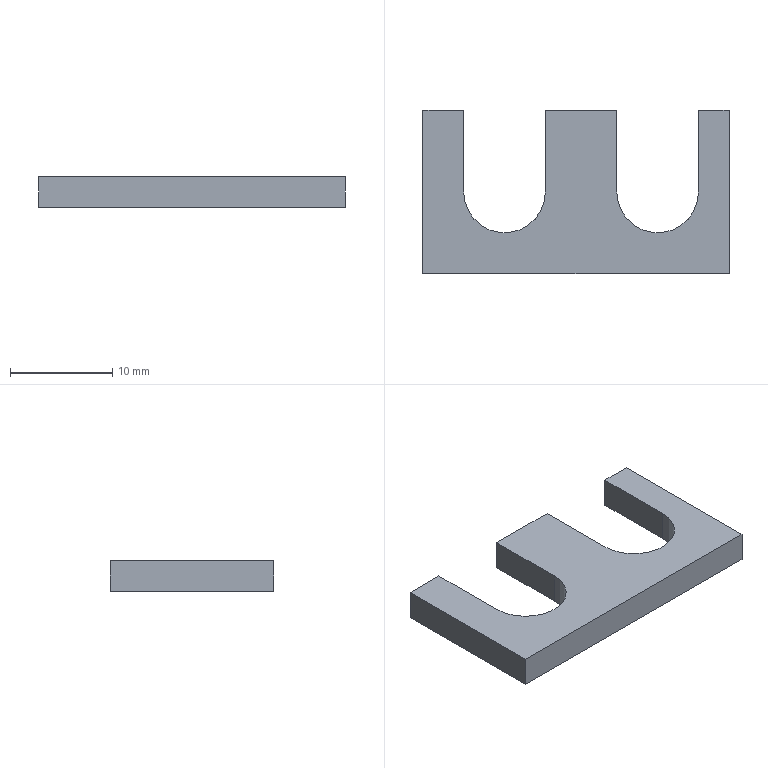Part | SolidWorks | features Extrusion 1 | 1 solid | 14 faces | box 30 x 16 x 3 mm | volume 905.204 mm3 | plane 12 | cylinder 2 | commonest cylinder face diameters 8 x2
STEP:
#1=CARTESIAN_POINT('',(0.,16.,0.));
#2=VERTEX_POINT('',#1);
#3=CARTESIAN_POINT('',(0.,0.,0.));
#4=VERTEX_POINT('',#3);
#5=CARTESIAN_POINT('',(0.,0.,0.));
#6=DIRECTION('',(0.,-1.,0.));
#7=VECTOR('',#6,1000.);
#8=LINE('',#5,#7);
#9=EDGE_CURVE('',#2,#4,#8,.T.);
#10=ORIENTED_EDGE('',*,*,#9,.T.);
#11=CARTESIAN_POINT('',(0.,0.,3.));
#12=VERTEX_POINT('',#11);
#13=CARTESIAN_POINT('',(0.,0.,3.));
#14=DIRECTION('',(0.,0.,-1.));
#15=VECTOR('',#14,1000.);
#16=LINE('',#13,#15);
#17=EDGE_CURVE('',#12,#4,#16,.T.);
#18=ORIENTED_EDGE('',*,*,#17,.F.);
#19=CARTESIAN_POINT('',(0.,16.,3.));
#20=VERTEX_POINT('',#19);
#21=CARTESIAN_POINT('',(0.,0.,3.));
#22=DIRECTION('',(0.,-1.,0.));
#23=VECTOR('',#22,1000.);
#24=LINE('',#21,#23);
#25=EDGE_CURVE('',#20,#12,#24,.T.);
#26=ORIENTED_EDGE('',*,*,#25,.F.);
#27=CARTESIAN_POINT('',(0.,16.,3.));
#28=DIRECTION('',(0.,0.,-1.));
#29=VECTOR('',#28,1000.);
#30=LINE('',#27,#29);
#31=EDGE_CURVE('',#20,#2,#30,.T.);
#32=ORIENTED_EDGE('',*,*,#31,.T.);
#33=EDGE_LOOP('',(#10,#18,#26,#32));
#34=FACE_OUTER_BOUND('',#33,.T.);
#35=CARTESIAN_POINT('',(0.,0.,3.));
#36=DIRECTION('',(1.,0.,0.));
#37=DIRECTION('',(0.,0.,-1.));
#38=AXIS2_PLACEMENT_3D('',#35,#36,#37);
#39=PLANE('',#38);
#40=ADVANCED_FACE('',(#34),#39,.F.);
#41=CARTESIAN_POINT('',(30.,0.,0.));
#42=VERTEX_POINT('',#41);
#43=CARTESIAN_POINT('',(0.,0.,0.));
#44=DIRECTION('',(1.,0.,0.));
#45=VECTOR('',#44,1000.);
#46=LINE('',#43,#45);
#47=EDGE_CURVE('',#4,#42,#46,.T.);
#48=ORIENTED_EDGE('',*,*,#47,.T.);
#49=CARTESIAN_POINT('',(30.,0.,3.));
#50=VERTEX_POINT('',#49);
#51=CARTESIAN_POINT('',(30.,0.,3.));
#52=DIRECTION('',(0.,0.,-1.));
#53=VECTOR('',#52,1000.);
#54=LINE('',#51,#53);
#55=EDGE_CURVE('',#50,#42,#54,.T.);
#56=ORIENTED_EDGE('',*,*,#55,.F.);
#57=CARTESIAN_POINT('',(0.,0.,3.));
#58=DIRECTION('',(1.,0.,0.));
#59=VECTOR('',#58,1000.);
#60=LINE('',#57,#59);
#61=EDGE_CURVE('',#12,#50,#60,.T.);
#62=ORIENTED_EDGE('',*,*,#61,.F.);
#63=ORIENTED_EDGE('',*,*,#17,.T.);
#64=EDGE_LOOP('',(#48,#56,#62,#63));
#65=FACE_OUTER_BOUND('',#64,.T.);
#66=CARTESIAN_POINT('',(0.,0.,3.));
#67=DIRECTION('',(0.,1.,0.));
#68=DIRECTION('',(0.,0.,1.));
#69=AXIS2_PLACEMENT_3D('',#66,#67,#68);
#70=PLANE('',#69);
#71=ADVANCED_FACE('',(#65),#70,.F.);
#72=CARTESIAN_POINT('',(30.,16.,0.));
#73=VERTEX_POINT('',#72);
#74=CARTESIAN_POINT('',(30.,0.,0.));
#75=DIRECTION('',(0.,1.,0.));
#76=VECTOR('',#75,1000.);
#77=LINE('',#74,#76);
#78=EDGE_CURVE('',#42,#73,#77,.T.);
#79=ORIENTED_EDGE('',*,*,#78,.T.);
#80=CARTESIAN_POINT('',(30.,16.,3.));
#81=VERTEX_POINT('',#80);
#82=CARTESIAN_POINT('',(30.,16.,3.));
#83=DIRECTION('',(0.,0.,-1.));
#84=VECTOR('',#83,1000.);
#85=LINE('',#82,#84);
#86=EDGE_CURVE('',#81,#73,#85,.T.);
#87=ORIENTED_EDGE('',*,*,#86,.F.);
#88=CARTESIAN_POINT('',(30.,0.,3.));
#89=DIRECTION('',(0.,1.,0.));
#90=VECTOR('',#89,1000.);
#91=LINE('',#88,#90);
#92=EDGE_CURVE('',#50,#81,#91,.T.);
#93=ORIENTED_EDGE('',*,*,#92,.F.);
#94=ORIENTED_EDGE('',*,*,#55,.T.);
#95=EDGE_LOOP('',(#79,#87,#93,#94));
#96=FACE_OUTER_BOUND('',#95,.T.);
#97=CARTESIAN_POINT('',(30.,0.,3.));
#98=DIRECTION('',(-1.,0.,0.));
#99=DIRECTION('',(0.,0.,1.));
#100=AXIS2_PLACEMENT_3D('',#97,#98,#99);
#101=PLANE('',#100);
#102=ADVANCED_FACE('',(#96),#101,.F.);
#103=CARTESIAN_POINT('',(27.,16.,0.));
#104=VERTEX_POINT('',#103);
#105=CARTESIAN_POINT('',(27.,16.,0.));
#106=DIRECTION('',(-1.,0.,0.));
#107=VECTOR('',#106,1000.);
#108=LINE('',#105,#107);
#109=EDGE_CURVE('',#73,#104,#108,.T.);
#110=ORIENTED_EDGE('',*,*,#109,.T.);
#111=CARTESIAN_POINT('',(27.,16.,3.));
#112=VERTEX_POINT('',#111);
#113=CARTESIAN_POINT('',(27.,16.,3.));
#114=DIRECTION('',(0.,0.,-1.));
#115=VECTOR('',#114,1000.);
#116=LINE('',#113,#115);
#117=EDGE_CURVE('',#112,#104,#116,.T.);
#118=ORIENTED_EDGE('',*,*,#117,.F.);
#119=CARTESIAN_POINT('',(27.,16.,3.));
#120=DIRECTION('',(-1.,0.,0.));
#121=VECTOR('',#120,1000.);
#122=LINE('',#119,#121);
#123=EDGE_CURVE('',#81,#112,#122,.T.);
#124=ORIENTED_EDGE('',*,*,#123,.F.);
#125=ORIENTED_EDGE('',*,*,#86,.T.);
#126=EDGE_LOOP('',(#110,#118,#124,#125));
#127=FACE_OUTER_BOUND('',#126,.T.);
#128=CARTESIAN_POINT('',(27.,16.,3.));
#129=DIRECTION('',(0.,-1.,0.));
#130=DIRECTION('',(0.,0.,-1.));
#131=AXIS2_PLACEMENT_3D('',#128,#129,#130);
#132=PLANE('',#131);
#133=ADVANCED_FACE('',(#127),#132,.F.);
#134=CARTESIAN_POINT('',(27.,8.,0.));
#135=VERTEX_POINT('',#134);
#136=CARTESIAN_POINT('',(27.,8.,0.));
#137=DIRECTION('',(0.,-1.,0.));
#138=VECTOR('',#137,1000.);
#139=LINE('',#136,#138);
#140=EDGE_CURVE('',#104,#135,#139,.T.);
#141=ORIENTED_EDGE('',*,*,#140,.T.);
#142=CARTESIAN_POINT('',(27.,8.,3.));
#143=VERTEX_POINT('',#142);
#144=CARTESIAN_POINT('',(27.,8.,3.));
#145=DIRECTION('',(0.,0.,-1.));
#146=VECTOR('',#145,1000.);
#147=LINE('',#144,#146);
#148=EDGE_CURVE('',#143,#135,#147,.T.);
#149=ORIENTED_EDGE('',*,*,#148,.F.);
#150=CARTESIAN_POINT('',(27.,8.,3.));
#151=DIRECTION('',(0.,-1.,0.));
#152=VECTOR('',#151,1000.);
#153=LINE('',#150,#152);
#154=EDGE_CURVE('',#112,#143,#153,.T.);
#155=ORIENTED_EDGE('',*,*,#154,.F.);
#156=ORIENTED_EDGE('',*,*,#117,.T.);
#157=EDGE_LOOP('',(#141,#149,#155,#156));
#158=FACE_OUTER_BOUND('',#157,.T.);
#159=CARTESIAN_POINT('',(27.,8.,3.));
#160=DIRECTION('',(1.,0.,0.));
#161=DIRECTION('',(0.,0.,-1.));
#162=AXIS2_PLACEMENT_3D('',#159,#160,#161);
#163=PLANE('',#162);
#164=ADVANCED_FACE('',(#158),#163,.F.);
#165=CARTESIAN_POINT('',(19.,8.,0.));
#166=VERTEX_POINT('',#165);
#167=CARTESIAN_POINT('',(23.,8.,0.));
#168=DIRECTION('',(0.,0.,-1.));
#169=DIRECTION('',(1.,0.,0.));
#170=AXIS2_PLACEMENT_3D('',#167,#168,#169);
#171=CIRCLE('',#170,4.);
#172=EDGE_CURVE('',#135,#166,#171,.T.);
#173=ORIENTED_EDGE('',*,*,#172,.T.);
#174=CARTESIAN_POINT('',(19.,8.,3.));
#175=VERTEX_POINT('',#174);
#176=CARTESIAN_POINT('',(19.,8.,3.));
#177=DIRECTION('',(0.,0.,-1.));
#178=VECTOR('',#177,1000.);
#179=LINE('',#176,#178);
#180=EDGE_CURVE('',#175,#166,#179,.T.);
#181=ORIENTED_EDGE('',*,*,#180,.F.);
#182=CARTESIAN_POINT('',(23.,8.,3.));
#183=DIRECTION('',(0.,0.,-1.));
#184=DIRECTION('',(1.,0.,0.));
#185=AXIS2_PLACEMENT_3D('',#182,#183,#184);
#186=CIRCLE('',#185,4.);
#187=EDGE_CURVE('',#143,#175,#186,.T.);
#188=ORIENTED_EDGE('',*,*,#187,.F.);
#189=ORIENTED_EDGE('',*,*,#148,.T.);
#190=EDGE_LOOP('',(#173,#181,#188,#189));
#191=FACE_OUTER_BOUND('',#190,.T.);
#192=CARTESIAN_POINT('',(23.,8.,3.));
#193=DIRECTION('',(0.,0.,-1.));
#194=DIRECTION('',(-1.,0.,0.));
#195=AXIS2_PLACEMENT_3D('',#192,#193,#194);
#196=CYLINDRICAL_SURFACE('',#195,4.);
#197=ADVANCED_FACE('',(#191),#196,.F.);
#198=CARTESIAN_POINT('',(19.,16.,0.));
#199=VERTEX_POINT('',#198);
#200=CARTESIAN_POINT('',(19.,8.,0.));
#201=DIRECTION('',(0.,1.,0.));
#202=VECTOR('',#201,1000.);
#203=LINE('',#200,#202);
#204=EDGE_CURVE('',#166,#199,#203,.T.);
#205=ORIENTED_EDGE('',*,*,#204,.T.);
#206=CARTESIAN_POINT('',(19.,16.,3.));
#207=VERTEX_POINT('',#206);
#208=CARTESIAN_POINT('',(19.,16.,3.));
#209=DIRECTION('',(0.,0.,-1.));
#210=VECTOR('',#209,1000.);
#211=LINE('',#208,#210);
#212=EDGE_CURVE('',#207,#199,#211,.T.);
#213=ORIENTED_EDGE('',*,*,#212,.F.);
#214=CARTESIAN_POINT('',(19.,8.,3.));
#215=DIRECTION('',(0.,1.,0.));
#216=VECTOR('',#215,1000.);
#217=LINE('',#214,#216);
#218=EDGE_CURVE('',#175,#207,#217,.T.);
#219=ORIENTED_EDGE('',*,*,#218,.F.);
#220=ORIENTED_EDGE('',*,*,#180,.T.);
#221=EDGE_LOOP('',(#205,#213,#219,#220));
#222=FACE_OUTER_BOUND('',#221,.T.);
#223=CARTESIAN_POINT('',(19.,8.,3.));
#224=DIRECTION('',(-1.,0.,0.));
#225=DIRECTION('',(0.,0.,1.));
#226=AXIS2_PLACEMENT_3D('',#223,#224,#225);
#227=PLANE('',#226);
#228=ADVANCED_FACE('',(#222),#227,.F.);
#229=CARTESIAN_POINT('',(12.,16.,0.));
#230=VERTEX_POINT('',#229);
#231=CARTESIAN_POINT('',(12.,16.,0.));
#232=DIRECTION('',(-1.,0.,0.));
#233=VECTOR('',#232,1000.);
#234=LINE('',#231,#233);
#235=EDGE_CURVE('',#199,#230,#234,.T.);
#236=ORIENTED_EDGE('',*,*,#235,.T.);
#237=CARTESIAN_POINT('',(12.,16.,3.));
#238=VERTEX_POINT('',#237);
#239=CARTESIAN_POINT('',(12.,16.,3.));
#240=DIRECTION('',(0.,0.,-1.));
#241=VECTOR('',#240,1000.);
#242=LINE('',#239,#241);
#243=EDGE_CURVE('',#238,#230,#242,.T.);
#244=ORIENTED_EDGE('',*,*,#243,.F.);
#245=CARTESIAN_POINT('',(12.,16.,3.));
#246=DIRECTION('',(-1.,0.,0.));
#247=VECTOR('',#246,1000.);
#248=LINE('',#245,#247);
#249=EDGE_CURVE('',#207,#238,#248,.T.);
#250=ORIENTED_EDGE('',*,*,#249,.F.);
#251=ORIENTED_EDGE('',*,*,#212,.T.);
#252=EDGE_LOOP('',(#236,#244,#250,#251));
#253=FACE_OUTER_BOUND('',#252,.T.);
#254=CARTESIAN_POINT('',(12.,16.,3.));
#255=DIRECTION('',(0.,-1.,0.));
#256=DIRECTION('',(0.,0.,-1.));
#257=AXIS2_PLACEMENT_3D('',#254,#255,#256);
#258=PLANE('',#257);
#259=ADVANCED_FACE('',(#253),#258,.F.);
#260=CARTESIAN_POINT('',(12.,8.,0.));
#261=VERTEX_POINT('',#260);
#262=CARTESIAN_POINT('',(12.,8.,0.));
#263=DIRECTION('',(0.,-1.,0.));
#264=VECTOR('',#263,1000.);
#265=LINE('',#262,#264);
#266=EDGE_CURVE('',#230,#261,#265,.T.);
#267=ORIENTED_EDGE('',*,*,#266,.T.);
#268=CARTESIAN_POINT('',(12.,8.,3.));
#269=VERTEX_POINT('',#268);
#270=CARTESIAN_POINT('',(12.,8.,3.));
#271=DIRECTION('',(0.,0.,-1.));
#272=VECTOR('',#271,1000.);
#273=LINE('',#270,#272);
#274=EDGE_CURVE('',#269,#261,#273,.T.);
#275=ORIENTED_EDGE('',*,*,#274,.F.);
#276=CARTESIAN_POINT('',(12.,8.,3.));
#277=DIRECTION('',(0.,-1.,0.));
#278=VECTOR('',#277,1000.);
#279=LINE('',#276,#278);
#280=EDGE_CURVE('',#238,#269,#279,.T.);
#281=ORIENTED_EDGE('',*,*,#280,.F.);
#282=ORIENTED_EDGE('',*,*,#243,.T.);
#283=EDGE_LOOP('',(#267,#275,#281,#282));
#284=FACE_OUTER_BOUND('',#283,.T.);
#285=CARTESIAN_POINT('',(12.,8.,3.));
#286=DIRECTION('',(1.,0.,0.));
#287=DIRECTION('',(0.,0.,-1.));
#288=AXIS2_PLACEMENT_3D('',#285,#286,#287);
#289=PLANE('',#288);
#290=ADVANCED_FACE('',(#284),#289,.F.);
#291=CARTESIAN_POINT('',(4.,8.,0.));
#292=VERTEX_POINT('',#291);
#293=CARTESIAN_POINT('',(8.,8.,0.));
#294=DIRECTION('',(0.,0.,-1.));
#295=DIRECTION('',(1.,0.,0.));
#296=AXIS2_PLACEMENT_3D('',#293,#294,#295);
#297=CIRCLE('',#296,4.);
#298=EDGE_CURVE('',#261,#292,#297,.T.);
#299=ORIENTED_EDGE('',*,*,#298,.T.);
#300=CARTESIAN_POINT('',(4.,8.,3.));
#301=VERTEX_POINT('',#300);
#302=CARTESIAN_POINT('',(4.,8.,3.));
#303=DIRECTION('',(0.,0.,-1.));
#304=VECTOR('',#303,1000.);
#305=LINE('',#302,#304);
#306=EDGE_CURVE('',#301,#292,#305,.T.);
#307=ORIENTED_EDGE('',*,*,#306,.F.);
#308=CARTESIAN_POINT('',(8.,8.,3.));
#309=DIRECTION('',(0.,0.,-1.));
#310=DIRECTION('',(1.,0.,0.));
#311=AXIS2_PLACEMENT_3D('',#308,#309,#310);
#312=CIRCLE('',#311,4.);
#313=EDGE_CURVE('',#269,#301,#312,.T.);
#314=ORIENTED_EDGE('',*,*,#313,.F.);
#315=ORIENTED_EDGE('',*,*,#274,.T.);
#316=EDGE_LOOP('',(#299,#307,#314,#315));
#317=FACE_OUTER_BOUND('',#316,.T.);
#318=CARTESIAN_POINT('',(8.,8.,3.));
#319=DIRECTION('',(0.,0.,-1.));
#320=DIRECTION('',(-1.,0.,0.));
#321=AXIS2_PLACEMENT_3D('',#318,#319,#320);
#322=CYLINDRICAL_SURFACE('',#321,4.);
#323=ADVANCED_FACE('',(#317),#322,.F.);
#324=CARTESIAN_POINT('',(4.,16.,0.));
#325=VERTEX_POINT('',#324);
#326=CARTESIAN_POINT('',(4.,8.,0.));
#327=DIRECTION('',(0.,1.,0.));
#328=VECTOR('',#327,1000.);
#329=LINE('',#326,#328);
#330=EDGE_CURVE('',#292,#325,#329,.T.);
#331=ORIENTED_EDGE('',*,*,#330,.T.);
#332=CARTESIAN_POINT('',(4.,16.,3.));
#333=VERTEX_POINT('',#332);
#334=CARTESIAN_POINT('',(4.,16.,3.));
#335=DIRECTION('',(0.,0.,-1.));
#336=VECTOR('',#335,1000.);
#337=LINE('',#334,#336);
#338=EDGE_CURVE('',#333,#325,#337,.T.);
#339=ORIENTED_EDGE('',*,*,#338,.F.);
#340=CARTESIAN_POINT('',(4.,8.,3.));
#341=DIRECTION('',(0.,1.,0.));
#342=VECTOR('',#341,1000.);
#343=LINE('',#340,#342);
#344=EDGE_CURVE('',#301,#333,#343,.T.);
#345=ORIENTED_EDGE('',*,*,#344,.F.);
#346=ORIENTED_EDGE('',*,*,#306,.T.);
#347=EDGE_LOOP('',(#331,#339,#345,#346));
#348=FACE_OUTER_BOUND('',#347,.T.);
#349=CARTESIAN_POINT('',(4.,8.,3.));
#350=DIRECTION('',(-1.,0.,0.));
#351=DIRECTION('',(0.,0.,1.));
#352=AXIS2_PLACEMENT_3D('',#349,#350,#351);
#353=PLANE('',#352);
#354=ADVANCED_FACE('',(#348),#353,.F.);
#355=CARTESIAN_POINT('',(0.,16.,0.));
#356=DIRECTION('',(-1.,0.,0.));
#357=VECTOR('',#356,1000.);
#358=LINE('',#355,#357);
#359=EDGE_CURVE('',#325,#2,#358,.T.);
#360=ORIENTED_EDGE('',*,*,#359,.T.);
#361=ORIENTED_EDGE('',*,*,#31,.F.);
#362=CARTESIAN_POINT('',(0.,16.,3.));
#363=DIRECTION('',(-1.,0.,0.));
#364=VECTOR('',#363,1000.);
#365=LINE('',#362,#364);
#366=EDGE_CURVE('',#333,#20,#365,.T.);
#367=ORIENTED_EDGE('',*,*,#366,.F.);
#368=ORIENTED_EDGE('',*,*,#338,.T.);
#369=EDGE_LOOP('',(#360,#361,#367,#368));
#370=FACE_OUTER_BOUND('',#369,.T.);
#371=CARTESIAN_POINT('',(0.,16.,3.));
#372=DIRECTION('',(0.,-1.,0.));
#373=DIRECTION('',(0.,0.,-1.));
#374=AXIS2_PLACEMENT_3D('',#371,#372,#373);
#375=PLANE('',#374);
#376=ADVANCED_FACE('',(#370),#375,.F.);
#377=ORIENTED_EDGE('',*,*,#25,.T.);
#378=ORIENTED_EDGE('',*,*,#61,.T.);
#379=ORIENTED_EDGE('',*,*,#92,.T.);
#380=ORIENTED_EDGE('',*,*,#123,.T.);
#381=ORIENTED_EDGE('',*,*,#154,.T.);
#382=ORIENTED_EDGE('',*,*,#187,.T.);
#383=ORIENTED_EDGE('',*,*,#218,.T.);
#384=ORIENTED_EDGE('',*,*,#249,.T.);
#385=ORIENTED_EDGE('',*,*,#280,.T.);
#386=ORIENTED_EDGE('',*,*,#313,.T.);
#387=ORIENTED_EDGE('',*,*,#344,.T.);
#388=ORIENTED_EDGE('',*,*,#366,.T.);
#389=EDGE_LOOP('',(#377,#378,#379,#380,#381,#382,#383,#384,#385,#386,#387,#388));
#390=FACE_OUTER_BOUND('',#389,.T.);
#391=CARTESIAN_POINT('',(8.,8.,3.));
#392=DIRECTION('',(0.,0.,1.));
#393=DIRECTION('',(1.,0.,0.));
#394=AXIS2_PLACEMENT_3D('',#391,#392,#393);
#395=PLANE('',#394);
#396=ADVANCED_FACE('',(#390),#395,.T.);
#397=ORIENTED_EDGE('',*,*,#9,.F.);
#398=ORIENTED_EDGE('',*,*,#359,.F.);
#399=ORIENTED_EDGE('',*,*,#330,.F.);
#400=ORIENTED_EDGE('',*,*,#298,.F.);
#401=ORIENTED_EDGE('',*,*,#266,.F.);
#402=ORIENTED_EDGE('',*,*,#235,.F.);
#403=ORIENTED_EDGE('',*,*,#204,.F.);
#404=ORIENTED_EDGE('',*,*,#172,.F.);
#405=ORIENTED_EDGE('',*,*,#140,.F.);
#406=ORIENTED_EDGE('',*,*,#109,.F.);
#407=ORIENTED_EDGE('',*,*,#78,.F.);
#408=ORIENTED_EDGE('',*,*,#47,.F.);
#409=EDGE_LOOP('',(#397,#398,#399,#400,#401,#402,#403,#404,#405,#406,#407,#408));
#410=FACE_OUTER_BOUND('',#409,.T.);
#411=CARTESIAN_POINT('',(8.,8.,0.));
#412=DIRECTION('',(0.,0.,1.));
#413=DIRECTION('',(1.,0.,0.));
#414=AXIS2_PLACEMENT_3D('',#411,#412,#413);
#415=PLANE('',#414);
#416=ADVANCED_FACE('',(#410),#415,.F.);
#417=CLOSED_SHELL('',(#40,#71,#102,#133,#164,#197,#228,#259,#290,#323,#354,#376,#396,#416));
#418=MANIFOLD_SOLID_BREP('',#417);
#419=CARTESIAN_POINT('',(0.,0.,0.));
#420=DIRECTION('',(0.,0.,1.));
#421=DIRECTION('',(1.,0.,0.));
#422=AXIS2_PLACEMENT_3D('',#419,#420,#421);
#423=(LENGTH_UNIT()NAMED_UNIT(*)SI_UNIT(.MILLI.,.METRE.));
#424=UNCERTAINTY_MEASURE_WITH_UNIT(LENGTH_MEASURE(0.00001),#423,'','');
#425=(NAMED_UNIT(*)PLANE_ANGLE_UNIT()SI_UNIT($,.RADIAN.));
#426=(NAMED_UNIT(*)SI_UNIT($,.STERADIAN.)SOLID_ANGLE_UNIT());
#427=(GEOMETRIC_REPRESENTATION_CONTEXT(3)GLOBAL_UNCERTAINTY_ASSIGNED_CONTEXT((#424))GLOBAL_UNIT_ASSIGNED_CONTEXT((#423,#425,#426))REPRESENTATION_CONTEXT('',''));
#428=ADVANCED_BREP_SHAPE_REPRESENTATION('',(#418,#422),#427);